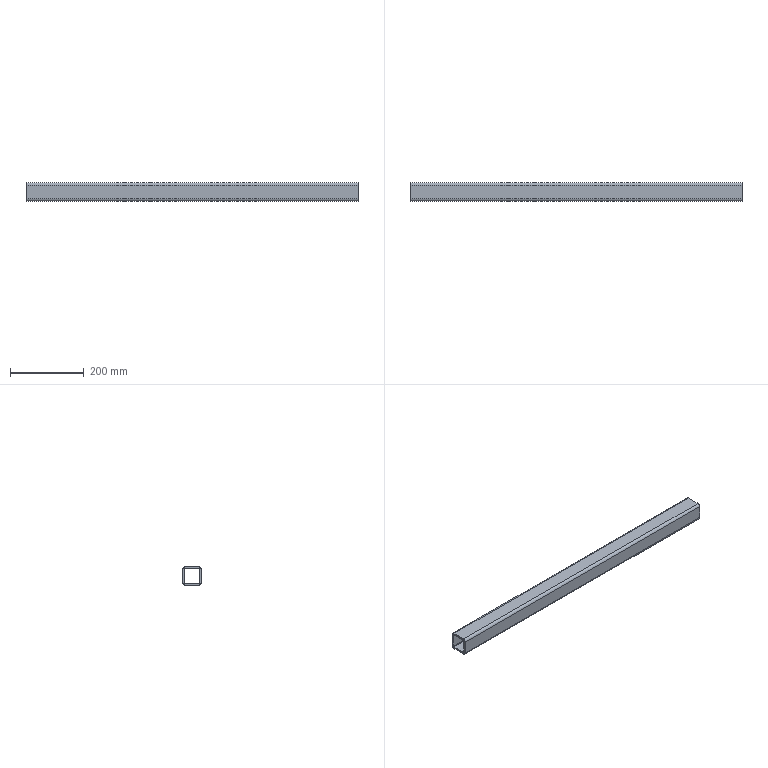Part | NX | 1 solid | 18 faces | box 900 x 50 x 50 mm | volume 775235 mm3 | plane 10 | cylinder 8 | commonest cylinder face diameters 4 x4 14 x4
STEP:
#1=CARTESIAN_POINT('',(-600.,179.,180.));
#2=VERTEX_POINT('',#1);
#3=CARTESIAN_POINT('',(300.,179.,180.));
#4=VERTEX_POINT('',#3);
#5=CARTESIAN_POINT('',(-625.,179.,180.));
#6=DIRECTION('',(1.,0.,0.));
#7=VECTOR('',#6,1000.);
#8=LINE('',#5,#7);
#9=EDGE_CURVE('',#2,#4,#8,.T.);
#10=ORIENTED_EDGE('',*,*,#9,.F.);
#11=CARTESIAN_POINT('',(-600.,143.,180.));
#12=VERTEX_POINT('',#11);
#13=CARTESIAN_POINT('',(-600.,143.,180.));
#14=DIRECTION('',(0.,-1.,0.));
#15=VECTOR('',#14,1000.);
#16=LINE('',#13,#15);
#17=EDGE_CURVE('',#2,#12,#16,.T.);
#18=ORIENTED_EDGE('',*,*,#17,.T.);
#19=CARTESIAN_POINT('',(300.,143.,180.));
#20=VERTEX_POINT('',#19);
#21=CARTESIAN_POINT('',(-625.,143.,180.));
#22=DIRECTION('',(1.,0.,0.));
#23=VECTOR('',#22,1000.);
#24=LINE('',#21,#23);
#25=EDGE_CURVE('',#12,#20,#24,.T.);
#26=ORIENTED_EDGE('',*,*,#25,.T.);
#27=CARTESIAN_POINT('',(300.,143.,180.));
#28=DIRECTION('',(0.,1.,0.));
#29=VECTOR('',#28,1000.);
#30=LINE('',#27,#29);
#31=EDGE_CURVE('',#20,#4,#30,.T.);
#32=ORIENTED_EDGE('',*,*,#31,.T.);
#33=EDGE_LOOP('',(#10,#18,#26,#32));
#34=FACE_BOUND('',#33,.T.);
#35=CARTESIAN_POINT('',(-625.,143.,180.));
#36=DIRECTION('',(0.,0.,1.));
#37=DIRECTION('',(1.,0.,0.));
#38=AXIS2_PLACEMENT_3D('',#35,#36,#37);
#39=PLANE('',#38);
#40=ADVANCED_FACE('',(#34),#39,.T.);
#41=ORIENTED_EDGE('',*,*,#25,.F.);
#42=CARTESIAN_POINT('',(-600.,141.,182.));
#43=VERTEX_POINT('',#42);
#44=CARTESIAN_POINT('',(-600.,143.,182.));
#45=DIRECTION('',(-1.,0.,0.));
#46=DIRECTION('',(0.,-1.,0.));
#47=AXIS2_PLACEMENT_3D('',#44,#45,#46);
#48=CIRCLE('',#47,2.);
#49=EDGE_CURVE('',#12,#43,#48,.T.);
#50=ORIENTED_EDGE('',*,*,#49,.T.);
#51=CARTESIAN_POINT('',(300.,141.,182.));
#52=VERTEX_POINT('',#51);
#53=CARTESIAN_POINT('',(-625.,141.,182.));
#54=DIRECTION('',(1.,0.,0.));
#55=VECTOR('',#54,1000.);
#56=LINE('',#53,#55);
#57=EDGE_CURVE('',#43,#52,#56,.T.);
#58=ORIENTED_EDGE('',*,*,#57,.T.);
#59=CARTESIAN_POINT('',(300.,143.,182.));
#60=DIRECTION('',(1.,0.,0.));
#61=DIRECTION('',(0.,1.,0.));
#62=AXIS2_PLACEMENT_3D('',#59,#60,#61);
#63=CIRCLE('',#62,2.);
#64=EDGE_CURVE('',#52,#20,#63,.T.);
#65=ORIENTED_EDGE('',*,*,#64,.T.);
#66=EDGE_LOOP('',(#41,#50,#58,#65));
#67=FACE_BOUND('',#66,.T.);
#68=CARTESIAN_POINT('',(-625.,143.,182.));
#69=DIRECTION('',(1.,0.,0.));
#70=DIRECTION('',(0.,0.,-1.));
#71=AXIS2_PLACEMENT_3D('',#68,#69,#70);
#72=CYLINDRICAL_SURFACE('',#71,2.);
#73=ADVANCED_FACE('',(#67),#72,.F.);
#74=ORIENTED_EDGE('',*,*,#57,.F.);
#75=CARTESIAN_POINT('',(-600.,141.,218.));
#76=VERTEX_POINT('',#75);
#77=CARTESIAN_POINT('',(-600.,141.,182.));
#78=DIRECTION('',(0.,0.,1.));
#79=VECTOR('',#78,1000.);
#80=LINE('',#77,#79);
#81=EDGE_CURVE('',#43,#76,#80,.T.);
#82=ORIENTED_EDGE('',*,*,#81,.T.);
#83=CARTESIAN_POINT('',(300.,141.,218.));
#84=VERTEX_POINT('',#83);
#85=CARTESIAN_POINT('',(-625.,141.,218.));
#86=DIRECTION('',(1.,0.,0.));
#87=VECTOR('',#86,1000.);
#88=LINE('',#85,#87);
#89=EDGE_CURVE('',#76,#84,#88,.T.);
#90=ORIENTED_EDGE('',*,*,#89,.T.);
#91=CARTESIAN_POINT('',(300.,141.,182.));
#92=DIRECTION('',(0.,0.,-1.));
#93=VECTOR('',#92,1000.);
#94=LINE('',#91,#93);
#95=EDGE_CURVE('',#84,#52,#94,.T.);
#96=ORIENTED_EDGE('',*,*,#95,.T.);
#97=EDGE_LOOP('',(#74,#82,#90,#96));
#98=FACE_BOUND('',#97,.T.);
#99=CARTESIAN_POINT('',(-625.,141.,182.));
#100=DIRECTION('',(0.,1.,0.));
#101=DIRECTION('',(0.,0.,1.));
#102=AXIS2_PLACEMENT_3D('',#99,#100,#101);
#103=PLANE('',#102);
#104=ADVANCED_FACE('',(#98),#103,.T.);
#105=ORIENTED_EDGE('',*,*,#89,.F.);
#106=CARTESIAN_POINT('',(-600.,143.,220.));
#107=VERTEX_POINT('',#106);
#108=CARTESIAN_POINT('',(-600.,143.,218.));
#109=DIRECTION('',(-1.,0.,0.));
#110=DIRECTION('',(0.,-1.,0.));
#111=AXIS2_PLACEMENT_3D('',#108,#109,#110);
#112=CIRCLE('',#111,2.);
#113=EDGE_CURVE('',#76,#107,#112,.T.);
#114=ORIENTED_EDGE('',*,*,#113,.T.);
#115=CARTESIAN_POINT('',(300.,143.,220.));
#116=VERTEX_POINT('',#115);
#117=CARTESIAN_POINT('',(-625.,143.,220.));
#118=DIRECTION('',(1.,0.,0.));
#119=VECTOR('',#118,1000.);
#120=LINE('',#117,#119);
#121=EDGE_CURVE('',#107,#116,#120,.T.);
#122=ORIENTED_EDGE('',*,*,#121,.T.);
#123=CARTESIAN_POINT('',(300.,143.,218.));
#124=DIRECTION('',(1.,0.,0.));
#125=DIRECTION('',(0.,1.,0.));
#126=AXIS2_PLACEMENT_3D('',#123,#124,#125);
#127=CIRCLE('',#126,2.);
#128=EDGE_CURVE('',#116,#84,#127,.T.);
#129=ORIENTED_EDGE('',*,*,#128,.T.);
#130=EDGE_LOOP('',(#105,#114,#122,#129));
#131=FACE_BOUND('',#130,.T.);
#132=CARTESIAN_POINT('',(-625.,143.,218.));
#133=DIRECTION('',(1.,0.,0.));
#134=DIRECTION('',(0.,0.,-1.));
#135=AXIS2_PLACEMENT_3D('',#132,#133,#134);
#136=CYLINDRICAL_SURFACE('',#135,2.);
#137=ADVANCED_FACE('',(#131),#136,.F.);
#138=ORIENTED_EDGE('',*,*,#121,.F.);
#139=CARTESIAN_POINT('',(-600.,179.,220.));
#140=VERTEX_POINT('',#139);
#141=CARTESIAN_POINT('',(-600.,179.,220.));
#142=DIRECTION('',(0.,1.,0.));
#143=VECTOR('',#142,1000.);
#144=LINE('',#141,#143);
#145=EDGE_CURVE('',#107,#140,#144,.T.);
#146=ORIENTED_EDGE('',*,*,#145,.T.);
#147=CARTESIAN_POINT('',(300.,179.,220.));
#148=VERTEX_POINT('',#147);
#149=CARTESIAN_POINT('',(-625.,179.,220.));
#150=DIRECTION('',(1.,0.,0.));
#151=VECTOR('',#150,1000.);
#152=LINE('',#149,#151);
#153=EDGE_CURVE('',#140,#148,#152,.T.);
#154=ORIENTED_EDGE('',*,*,#153,.T.);
#155=CARTESIAN_POINT('',(300.,179.,220.));
#156=DIRECTION('',(0.,-1.,0.));
#157=VECTOR('',#156,1000.);
#158=LINE('',#155,#157);
#159=EDGE_CURVE('',#148,#116,#158,.T.);
#160=ORIENTED_EDGE('',*,*,#159,.T.);
#161=EDGE_LOOP('',(#138,#146,#154,#160));
#162=FACE_BOUND('',#161,.T.);
#163=CARTESIAN_POINT('',(-625.,179.,220.));
#164=DIRECTION('',(0.,0.,-1.));
#165=DIRECTION('',(-1.,0.,0.));
#166=AXIS2_PLACEMENT_3D('',#163,#164,#165);
#167=PLANE('',#166);
#168=ADVANCED_FACE('',(#162),#167,.T.);
#169=ORIENTED_EDGE('',*,*,#153,.F.);
#170=CARTESIAN_POINT('',(-600.,181.,218.));
#171=VERTEX_POINT('',#170);
#172=CARTESIAN_POINT('',(-600.,179.,218.));
#173=DIRECTION('',(-1.,0.,0.));
#174=DIRECTION('',(0.,-1.,0.));
#175=AXIS2_PLACEMENT_3D('',#172,#173,#174);
#176=CIRCLE('',#175,2.);
#177=EDGE_CURVE('',#140,#171,#176,.T.);
#178=ORIENTED_EDGE('',*,*,#177,.T.);
#179=CARTESIAN_POINT('',(300.,181.,218.));
#180=VERTEX_POINT('',#179);
#181=CARTESIAN_POINT('',(-625.,181.,218.));
#182=DIRECTION('',(1.,0.,0.));
#183=VECTOR('',#182,1000.);
#184=LINE('',#181,#183);
#185=EDGE_CURVE('',#171,#180,#184,.T.);
#186=ORIENTED_EDGE('',*,*,#185,.T.);
#187=CARTESIAN_POINT('',(300.,179.,218.));
#188=DIRECTION('',(1.,0.,0.));
#189=DIRECTION('',(0.,1.,0.));
#190=AXIS2_PLACEMENT_3D('',#187,#188,#189);
#191=CIRCLE('',#190,2.);
#192=EDGE_CURVE('',#180,#148,#191,.T.);
#193=ORIENTED_EDGE('',*,*,#192,.T.);
#194=EDGE_LOOP('',(#169,#178,#186,#193));
#195=FACE_BOUND('',#194,.T.);
#196=CARTESIAN_POINT('',(-625.,179.,218.));
#197=DIRECTION('',(1.,0.,0.));
#198=DIRECTION('',(0.,0.,-1.));
#199=AXIS2_PLACEMENT_3D('',#196,#197,#198);
#200=CYLINDRICAL_SURFACE('',#199,2.);
#201=ADVANCED_FACE('',(#195),#200,.F.);
#202=ORIENTED_EDGE('',*,*,#185,.F.);
#203=CARTESIAN_POINT('',(-600.,181.,182.));
#204=VERTEX_POINT('',#203);
#205=CARTESIAN_POINT('',(-600.,181.,218.));
#206=DIRECTION('',(0.,0.,-1.));
#207=VECTOR('',#206,1000.);
#208=LINE('',#205,#207);
#209=EDGE_CURVE('',#171,#204,#208,.T.);
#210=ORIENTED_EDGE('',*,*,#209,.T.);
#211=CARTESIAN_POINT('',(300.,181.,182.));
#212=VERTEX_POINT('',#211);
#213=CARTESIAN_POINT('',(-625.,181.,182.));
#214=DIRECTION('',(1.,0.,0.));
#215=VECTOR('',#214,1000.);
#216=LINE('',#213,#215);
#217=EDGE_CURVE('',#204,#212,#216,.T.);
#218=ORIENTED_EDGE('',*,*,#217,.T.);
#219=CARTESIAN_POINT('',(300.,181.,218.));
#220=DIRECTION('',(0.,0.,1.));
#221=VECTOR('',#220,1000.);
#222=LINE('',#219,#221);
#223=EDGE_CURVE('',#212,#180,#222,.T.);
#224=ORIENTED_EDGE('',*,*,#223,.T.);
#225=EDGE_LOOP('',(#202,#210,#218,#224));
#226=FACE_BOUND('',#225,.T.);
#227=CARTESIAN_POINT('',(-625.,181.,218.));
#228=DIRECTION('',(0.,-1.,0.));
#229=DIRECTION('',(0.,0.,-1.));
#230=AXIS2_PLACEMENT_3D('',#227,#228,#229);
#231=PLANE('',#230);
#232=ADVANCED_FACE('',(#226),#231,.T.);
#233=ORIENTED_EDGE('',*,*,#217,.F.);
#234=CARTESIAN_POINT('',(-600.,179.,182.));
#235=DIRECTION('',(-1.,0.,0.));
#236=DIRECTION('',(0.,-1.,0.));
#237=AXIS2_PLACEMENT_3D('',#234,#235,#236);
#238=CIRCLE('',#237,2.);
#239=EDGE_CURVE('',#204,#2,#238,.T.);
#240=ORIENTED_EDGE('',*,*,#239,.T.);
#241=ORIENTED_EDGE('',*,*,#9,.T.);
#242=CARTESIAN_POINT('',(300.,179.,182.));
#243=DIRECTION('',(1.,0.,0.));
#244=DIRECTION('',(0.,1.,0.));
#245=AXIS2_PLACEMENT_3D('',#242,#243,#244);
#246=CIRCLE('',#245,2.);
#247=EDGE_CURVE('',#4,#212,#246,.T.);
#248=ORIENTED_EDGE('',*,*,#247,.T.);
#249=EDGE_LOOP('',(#233,#240,#241,#248));
#250=FACE_BOUND('',#249,.T.);
#251=CARTESIAN_POINT('',(-625.,179.,182.));
#252=DIRECTION('',(1.,0.,0.));
#253=DIRECTION('',(0.,0.,-1.));
#254=AXIS2_PLACEMENT_3D('',#251,#252,#253);
#255=CYLINDRICAL_SURFACE('',#254,2.);
#256=ADVANCED_FACE('',(#250),#255,.F.);
#257=CARTESIAN_POINT('',(-600.,143.,225.));
#258=VERTEX_POINT('',#257);
#259=CARTESIAN_POINT('',(-600.,179.,225.));
#260=VERTEX_POINT('',#259);
#261=CARTESIAN_POINT('',(-600.,0.,225.));
#262=DIRECTION('',(0.,1.,0.));
#263=VECTOR('',#262,1000.);
#264=LINE('',#261,#263);
#265=EDGE_CURVE('',#258,#260,#264,.T.);
#266=ORIENTED_EDGE('',*,*,#265,.F.);
#267=CARTESIAN_POINT('',(300.,143.,225.));
#268=VERTEX_POINT('',#267);
#269=CARTESIAN_POINT('',(-625.,143.,225.));
#270=DIRECTION('',(1.,0.,0.));
#271=VECTOR('',#270,1000.);
#272=LINE('',#269,#271);
#273=EDGE_CURVE('',#258,#268,#272,.T.);
#274=ORIENTED_EDGE('',*,*,#273,.T.);
#275=CARTESIAN_POINT('',(300.,179.,225.));
#276=VERTEX_POINT('',#275);
#277=CARTESIAN_POINT('',(300.,179.,225.));
#278=DIRECTION('',(0.,-1.,0.));
#279=VECTOR('',#278,1000.);
#280=LINE('',#277,#279);
#281=EDGE_CURVE('',#276,#268,#280,.T.);
#282=ORIENTED_EDGE('',*,*,#281,.F.);
#283=CARTESIAN_POINT('',(-625.,179.,225.));
#284=DIRECTION('',(1.,0.,0.));
#285=VECTOR('',#284,1000.);
#286=LINE('',#283,#285);
#287=EDGE_CURVE('',#260,#276,#286,.T.);
#288=ORIENTED_EDGE('',*,*,#287,.F.);
#289=EDGE_LOOP('',(#266,#274,#282,#288));
#290=FACE_BOUND('',#289,.T.);
#291=CARTESIAN_POINT('',(-625.,179.,225.));
#292=DIRECTION('',(0.,0.,-1.));
#293=DIRECTION('',(-1.,0.,0.));
#294=AXIS2_PLACEMENT_3D('',#291,#292,#293);
#295=PLANE('',#294);
#296=ADVANCED_FACE('',(#290),#295,.F.);
#297=CARTESIAN_POINT('',(-600.,136.,218.));
#298=VERTEX_POINT('',#297);
#299=CARTESIAN_POINT('',(-600.,143.,218.));
#300=DIRECTION('',(-1.,0.,0.));
#301=DIRECTION('',(0.,-1.,0.));
#302=AXIS2_PLACEMENT_3D('',#299,#300,#301);
#303=CIRCLE('',#302,7.);
#304=EDGE_CURVE('',#298,#258,#303,.T.);
#305=ORIENTED_EDGE('',*,*,#304,.F.);
#306=CARTESIAN_POINT('',(300.,136.,218.));
#307=VERTEX_POINT('',#306);
#308=CARTESIAN_POINT('',(-625.,136.,218.));
#309=DIRECTION('',(1.,0.,0.));
#310=VECTOR('',#309,1000.);
#311=LINE('',#308,#310);
#312=EDGE_CURVE('',#298,#307,#311,.T.);
#313=ORIENTED_EDGE('',*,*,#312,.T.);
#314=CARTESIAN_POINT('',(300.,143.,218.));
#315=DIRECTION('',(1.,0.,0.));
#316=DIRECTION('',(0.,1.,0.));
#317=AXIS2_PLACEMENT_3D('',#314,#315,#316);
#318=CIRCLE('',#317,7.);
#319=EDGE_CURVE('',#268,#307,#318,.T.);
#320=ORIENTED_EDGE('',*,*,#319,.F.);
#321=ORIENTED_EDGE('',*,*,#273,.F.);
#322=EDGE_LOOP('',(#305,#313,#320,#321));
#323=FACE_BOUND('',#322,.T.);
#324=CARTESIAN_POINT('',(-625.,143.,218.));
#325=DIRECTION('',(1.,0.,0.));
#326=DIRECTION('',(0.,0.,-1.));
#327=AXIS2_PLACEMENT_3D('',#324,#325,#326);
#328=CYLINDRICAL_SURFACE('',#327,7.);
#329=ADVANCED_FACE('',(#323),#328,.T.);
#330=CARTESIAN_POINT('',(-600.,136.,182.));
#331=VERTEX_POINT('',#330);
#332=CARTESIAN_POINT('',(-600.,136.,182.));
#333=DIRECTION('',(0.,0.,1.));
#334=VECTOR('',#333,1000.);
#335=LINE('',#332,#334);
#336=EDGE_CURVE('',#331,#298,#335,.T.);
#337=ORIENTED_EDGE('',*,*,#336,.F.);
#338=CARTESIAN_POINT('',(300.,136.,182.));
#339=VERTEX_POINT('',#338);
#340=CARTESIAN_POINT('',(-625.,136.,182.));
#341=DIRECTION('',(1.,0.,0.));
#342=VECTOR('',#341,1000.);
#343=LINE('',#340,#342);
#344=EDGE_CURVE('',#331,#339,#343,.T.);
#345=ORIENTED_EDGE('',*,*,#344,.T.);
#346=CARTESIAN_POINT('',(300.,136.,375.));
#347=DIRECTION('',(0.,0.,-1.));
#348=VECTOR('',#347,1000.);
#349=LINE('',#346,#348);
#350=EDGE_CURVE('',#307,#339,#349,.T.);
#351=ORIENTED_EDGE('',*,*,#350,.F.);
#352=ORIENTED_EDGE('',*,*,#312,.F.);
#353=EDGE_LOOP('',(#337,#345,#351,#352));
#354=FACE_BOUND('',#353,.T.);
#355=CARTESIAN_POINT('',(-625.,136.,182.));
#356=DIRECTION('',(0.,1.,0.));
#357=DIRECTION('',(0.,0.,1.));
#358=AXIS2_PLACEMENT_3D('',#355,#356,#357);
#359=PLANE('',#358);
#360=ADVANCED_FACE('',(#354),#359,.F.);
#361=CARTESIAN_POINT('',(-600.,143.,175.));
#362=VERTEX_POINT('',#361);
#363=CARTESIAN_POINT('',(-600.,143.,182.));
#364=DIRECTION('',(-1.,0.,0.));
#365=DIRECTION('',(0.,-1.,0.));
#366=AXIS2_PLACEMENT_3D('',#363,#364,#365);
#367=CIRCLE('',#366,7.);
#368=EDGE_CURVE('',#362,#331,#367,.T.);
#369=ORIENTED_EDGE('',*,*,#368,.F.);
#370=CARTESIAN_POINT('',(300.,143.,175.));
#371=VERTEX_POINT('',#370);
#372=CARTESIAN_POINT('',(-625.,143.,175.));
#373=DIRECTION('',(1.,0.,0.));
#374=VECTOR('',#373,1000.);
#375=LINE('',#372,#374);
#376=EDGE_CURVE('',#362,#371,#375,.T.);
#377=ORIENTED_EDGE('',*,*,#376,.T.);
#378=CARTESIAN_POINT('',(300.,143.,182.));
#379=DIRECTION('',(1.,0.,0.));
#380=DIRECTION('',(0.,1.,0.));
#381=AXIS2_PLACEMENT_3D('',#378,#379,#380);
#382=CIRCLE('',#381,7.);
#383=EDGE_CURVE('',#339,#371,#382,.T.);
#384=ORIENTED_EDGE('',*,*,#383,.F.);
#385=ORIENTED_EDGE('',*,*,#344,.F.);
#386=EDGE_LOOP('',(#369,#377,#384,#385));
#387=FACE_BOUND('',#386,.T.);
#388=CARTESIAN_POINT('',(-625.,143.,182.));
#389=DIRECTION('',(1.,0.,0.));
#390=DIRECTION('',(0.,0.,-1.));
#391=AXIS2_PLACEMENT_3D('',#388,#389,#390);
#392=CYLINDRICAL_SURFACE('',#391,7.);
#393=ADVANCED_FACE('',(#387),#392,.T.);
#394=CARTESIAN_POINT('',(-600.,179.,175.));
#395=VERTEX_POINT('',#394);
#396=CARTESIAN_POINT('',(-600.,0.,175.));
#397=DIRECTION('',(0.,1.,0.));
#398=VECTOR('',#397,1000.);
#399=LINE('',#396,#398);
#400=EDGE_CURVE('',#362,#395,#399,.T.);
#401=ORIENTED_EDGE('',*,*,#400,.T.);
#402=CARTESIAN_POINT('',(300.,179.,175.));
#403=VERTEX_POINT('',#402);
#404=CARTESIAN_POINT('',(-625.,179.,175.));
#405=DIRECTION('',(1.,0.,0.));
#406=VECTOR('',#405,1000.);
#407=LINE('',#404,#406);
#408=EDGE_CURVE('',#395,#403,#407,.T.);
#409=ORIENTED_EDGE('',*,*,#408,.T.);
#410=CARTESIAN_POINT('',(300.,143.,175.));
#411=DIRECTION('',(0.,1.,0.));
#412=VECTOR('',#411,1000.);
#413=LINE('',#410,#412);
#414=EDGE_CURVE('',#371,#403,#413,.T.);
#415=ORIENTED_EDGE('',*,*,#414,.F.);
#416=ORIENTED_EDGE('',*,*,#376,.F.);
#417=EDGE_LOOP('',(#401,#409,#415,#416));
#418=FACE_BOUND('',#417,.T.);
#419=CARTESIAN_POINT('',(-625.,143.,175.));
#420=DIRECTION('',(0.,0.,1.));
#421=DIRECTION('',(1.,0.,0.));
#422=AXIS2_PLACEMENT_3D('',#419,#420,#421);
#423=PLANE('',#422);
#424=ADVANCED_FACE('',(#418),#423,.F.);
#425=CARTESIAN_POINT('',(-600.,186.,182.));
#426=VERTEX_POINT('',#425);
#427=CARTESIAN_POINT('',(-600.,179.,182.));
#428=DIRECTION('',(-1.,0.,0.));
#429=DIRECTION('',(0.,-1.,0.));
#430=AXIS2_PLACEMENT_3D('',#427,#428,#429);
#431=CIRCLE('',#430,7.);
#432=EDGE_CURVE('',#426,#395,#431,.T.);
#433=ORIENTED_EDGE('',*,*,#432,.F.);
#434=CARTESIAN_POINT('',(300.,186.,182.));
#435=VERTEX_POINT('',#434);
#436=CARTESIAN_POINT('',(-625.,186.,182.));
#437=DIRECTION('',(1.,0.,0.));
#438=VECTOR('',#437,1000.);
#439=LINE('',#436,#438);
#440=EDGE_CURVE('',#426,#435,#439,.T.);
#441=ORIENTED_EDGE('',*,*,#440,.T.);
#442=CARTESIAN_POINT('',(300.,179.,182.));
#443=DIRECTION('',(1.,0.,0.));
#444=DIRECTION('',(0.,1.,0.));
#445=AXIS2_PLACEMENT_3D('',#442,#443,#444);
#446=CIRCLE('',#445,7.);
#447=EDGE_CURVE('',#403,#435,#446,.T.);
#448=ORIENTED_EDGE('',*,*,#447,.F.);
#449=ORIENTED_EDGE('',*,*,#408,.F.);
#450=EDGE_LOOP('',(#433,#441,#448,#449));
#451=FACE_BOUND('',#450,.T.);
#452=CARTESIAN_POINT('',(-625.,179.,182.));
#453=DIRECTION('',(1.,0.,0.));
#454=DIRECTION('',(0.,0.,-1.));
#455=AXIS2_PLACEMENT_3D('',#452,#453,#454);
#456=CYLINDRICAL_SURFACE('',#455,7.);
#457=ADVANCED_FACE('',(#451),#456,.T.);
#458=CARTESIAN_POINT('',(-600.,186.,218.));
#459=VERTEX_POINT('',#458);
#460=CARTESIAN_POINT('',(-600.,186.,218.));
#461=DIRECTION('',(0.,0.,-1.));
#462=VECTOR('',#461,1000.);
#463=LINE('',#460,#462);
#464=EDGE_CURVE('',#459,#426,#463,.T.);
#465=ORIENTED_EDGE('',*,*,#464,.F.);
#466=CARTESIAN_POINT('',(300.,186.,218.));
#467=VERTEX_POINT('',#466);
#468=CARTESIAN_POINT('',(-625.,186.,218.));
#469=DIRECTION('',(1.,0.,0.));
#470=VECTOR('',#469,1000.);
#471=LINE('',#468,#470);
#472=EDGE_CURVE('',#459,#467,#471,.T.);
#473=ORIENTED_EDGE('',*,*,#472,.T.);
#474=CARTESIAN_POINT('',(300.,186.,375.));
#475=DIRECTION('',(0.,0.,-1.));
#476=VECTOR('',#475,1000.);
#477=LINE('',#474,#476);
#478=EDGE_CURVE('',#467,#435,#477,.T.);
#479=ORIENTED_EDGE('',*,*,#478,.T.);
#480=ORIENTED_EDGE('',*,*,#440,.F.);
#481=EDGE_LOOP('',(#465,#473,#479,#480));
#482=FACE_BOUND('',#481,.T.);
#483=CARTESIAN_POINT('',(-625.,186.,218.));
#484=DIRECTION('',(0.,-1.,0.));
#485=DIRECTION('',(0.,0.,-1.));
#486=AXIS2_PLACEMENT_3D('',#483,#484,#485);
#487=PLANE('',#486);
#488=ADVANCED_FACE('',(#482),#487,.F.);
#489=CARTESIAN_POINT('',(-600.,179.,218.));
#490=DIRECTION('',(-1.,0.,0.));
#491=DIRECTION('',(0.,-1.,0.));
#492=AXIS2_PLACEMENT_3D('',#489,#490,#491);
#493=CIRCLE('',#492,7.);
#494=EDGE_CURVE('',#260,#459,#493,.T.);
#495=ORIENTED_EDGE('',*,*,#494,.F.);
#496=ORIENTED_EDGE('',*,*,#287,.T.);
#497=CARTESIAN_POINT('',(300.,179.,218.));
#498=DIRECTION('',(1.,0.,0.));
#499=DIRECTION('',(0.,1.,0.));
#500=AXIS2_PLACEMENT_3D('',#497,#498,#499);
#501=CIRCLE('',#500,7.);
#502=EDGE_CURVE('',#467,#276,#501,.T.);
#503=ORIENTED_EDGE('',*,*,#502,.F.);
#504=ORIENTED_EDGE('',*,*,#472,.F.);
#505=EDGE_LOOP('',(#495,#496,#503,#504));
#506=FACE_BOUND('',#505,.T.);
#507=CARTESIAN_POINT('',(-625.,179.,218.));
#508=DIRECTION('',(1.,0.,0.));
#509=DIRECTION('',(0.,0.,-1.));
#510=AXIS2_PLACEMENT_3D('',#507,#508,#509);
#511=CYLINDRICAL_SURFACE('',#510,7.);
#512=ADVANCED_FACE('',(#506),#511,.T.);
#513=ORIENTED_EDGE('',*,*,#31,.F.);
#514=ORIENTED_EDGE('',*,*,#64,.F.);
#515=ORIENTED_EDGE('',*,*,#95,.F.);
#516=ORIENTED_EDGE('',*,*,#128,.F.);
#517=ORIENTED_EDGE('',*,*,#159,.F.);
#518=ORIENTED_EDGE('',*,*,#192,.F.);
#519=ORIENTED_EDGE('',*,*,#223,.F.);
#520=ORIENTED_EDGE('',*,*,#247,.F.);
#521=EDGE_LOOP('',(#513,#514,#515,#516,#517,#518,#519,#520));
#522=FACE_BOUND('',#521,.T.);
#523=ORIENTED_EDGE('',*,*,#447,.T.);
#524=ORIENTED_EDGE('',*,*,#478,.F.);
#525=ORIENTED_EDGE('',*,*,#502,.T.);
#526=ORIENTED_EDGE('',*,*,#281,.T.);
#527=ORIENTED_EDGE('',*,*,#319,.T.);
#528=ORIENTED_EDGE('',*,*,#350,.T.);
#529=ORIENTED_EDGE('',*,*,#383,.T.);
#530=ORIENTED_EDGE('',*,*,#414,.T.);
#531=EDGE_LOOP('',(#523,#524,#525,#526,#527,#528,#529,#530));
#532=FACE_BOUND('',#531,.T.);
#533=CARTESIAN_POINT('',(300.,143.,375.));
#534=DIRECTION('',(1.,0.,0.));
#535=DIRECTION('',(0.,1.,0.));
#536=AXIS2_PLACEMENT_3D('',#533,#534,#535);
#537=PLANE('',#536);
#538=ADVANCED_FACE('',(#522,#532),#537,.T.);
#539=ORIENTED_EDGE('',*,*,#239,.F.);
#540=ORIENTED_EDGE('',*,*,#209,.F.);
#541=ORIENTED_EDGE('',*,*,#177,.F.);
#542=ORIENTED_EDGE('',*,*,#145,.F.);
#543=ORIENTED_EDGE('',*,*,#113,.F.);
#544=ORIENTED_EDGE('',*,*,#81,.F.);
#545=ORIENTED_EDGE('',*,*,#49,.F.);
#546=ORIENTED_EDGE('',*,*,#17,.F.);
#547=EDGE_LOOP('',(#539,#540,#541,#542,#543,#544,#545,#546));
#548=FACE_BOUND('',#547,.T.);
#549=ORIENTED_EDGE('',*,*,#304,.T.);
#550=ORIENTED_EDGE('',*,*,#265,.T.);
#551=ORIENTED_EDGE('',*,*,#494,.T.);
#552=ORIENTED_EDGE('',*,*,#464,.T.);
#553=ORIENTED_EDGE('',*,*,#432,.T.);
#554=ORIENTED_EDGE('',*,*,#400,.F.);
#555=ORIENTED_EDGE('',*,*,#368,.T.);
#556=ORIENTED_EDGE('',*,*,#336,.T.);
#557=EDGE_LOOP('',(#549,#550,#551,#552,#553,#554,#555,#556));
#558=FACE_BOUND('',#557,.T.);
#559=CARTESIAN_POINT('',(-600.,0.,218.));
#560=DIRECTION('',(-1.,0.,0.));
#561=DIRECTION('',(0.,-1.,0.));
#562=AXIS2_PLACEMENT_3D('',#559,#560,#561);
#563=PLANE('',#562);
#564=ADVANCED_FACE('',(#548,#558),#563,.T.);
#565=CLOSED_SHELL('',(#40,#73,#104,#137,#168,#201,#232,#256,#296,#329,#360,#393,#424,#457,#488,#512,#538,#564));
#566=MANIFOLD_SOLID_BREP('',#565);
#567=(LENGTH_UNIT()NAMED_UNIT(*)SI_UNIT(.MILLI.,.METRE.));
#568=UNCERTAINTY_MEASURE_WITH_UNIT(LENGTH_MEASURE(0.00001),#567,'','');
#569=(NAMED_UNIT(*)PLANE_ANGLE_UNIT()SI_UNIT($,.RADIAN.));
#570=(NAMED_UNIT(*)SI_UNIT($,.STERADIAN.)SOLID_ANGLE_UNIT());
#571=(GEOMETRIC_REPRESENTATION_CONTEXT(3)GLOBAL_UNCERTAINTY_ASSIGNED_CONTEXT((#568))GLOBAL_UNIT_ASSIGNED_CONTEXT((#567,#569,#570))REPRESENTATION_CONTEXT('',''));
#572=ADVANCED_BREP_SHAPE_REPRESENTATION('',(#566),#571);